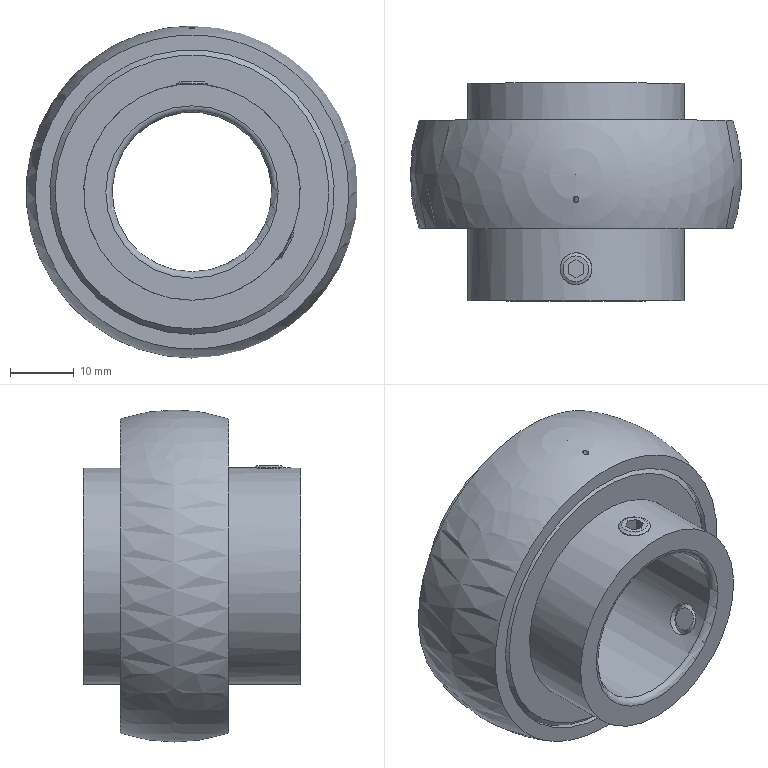Part | STEP file | 02288023_01 | 1 solid | 89 faces | box 52 x 34.1 x 52 mm | volume 26844 mm3 | plane 28 | torus 26 | cylinder 16 | sphere 13 | cone 6 | commonest cylinder face diameters 5 x4 44.547 x4 33.9 x2 33.92 x2 43.674 x2 0.885 x1